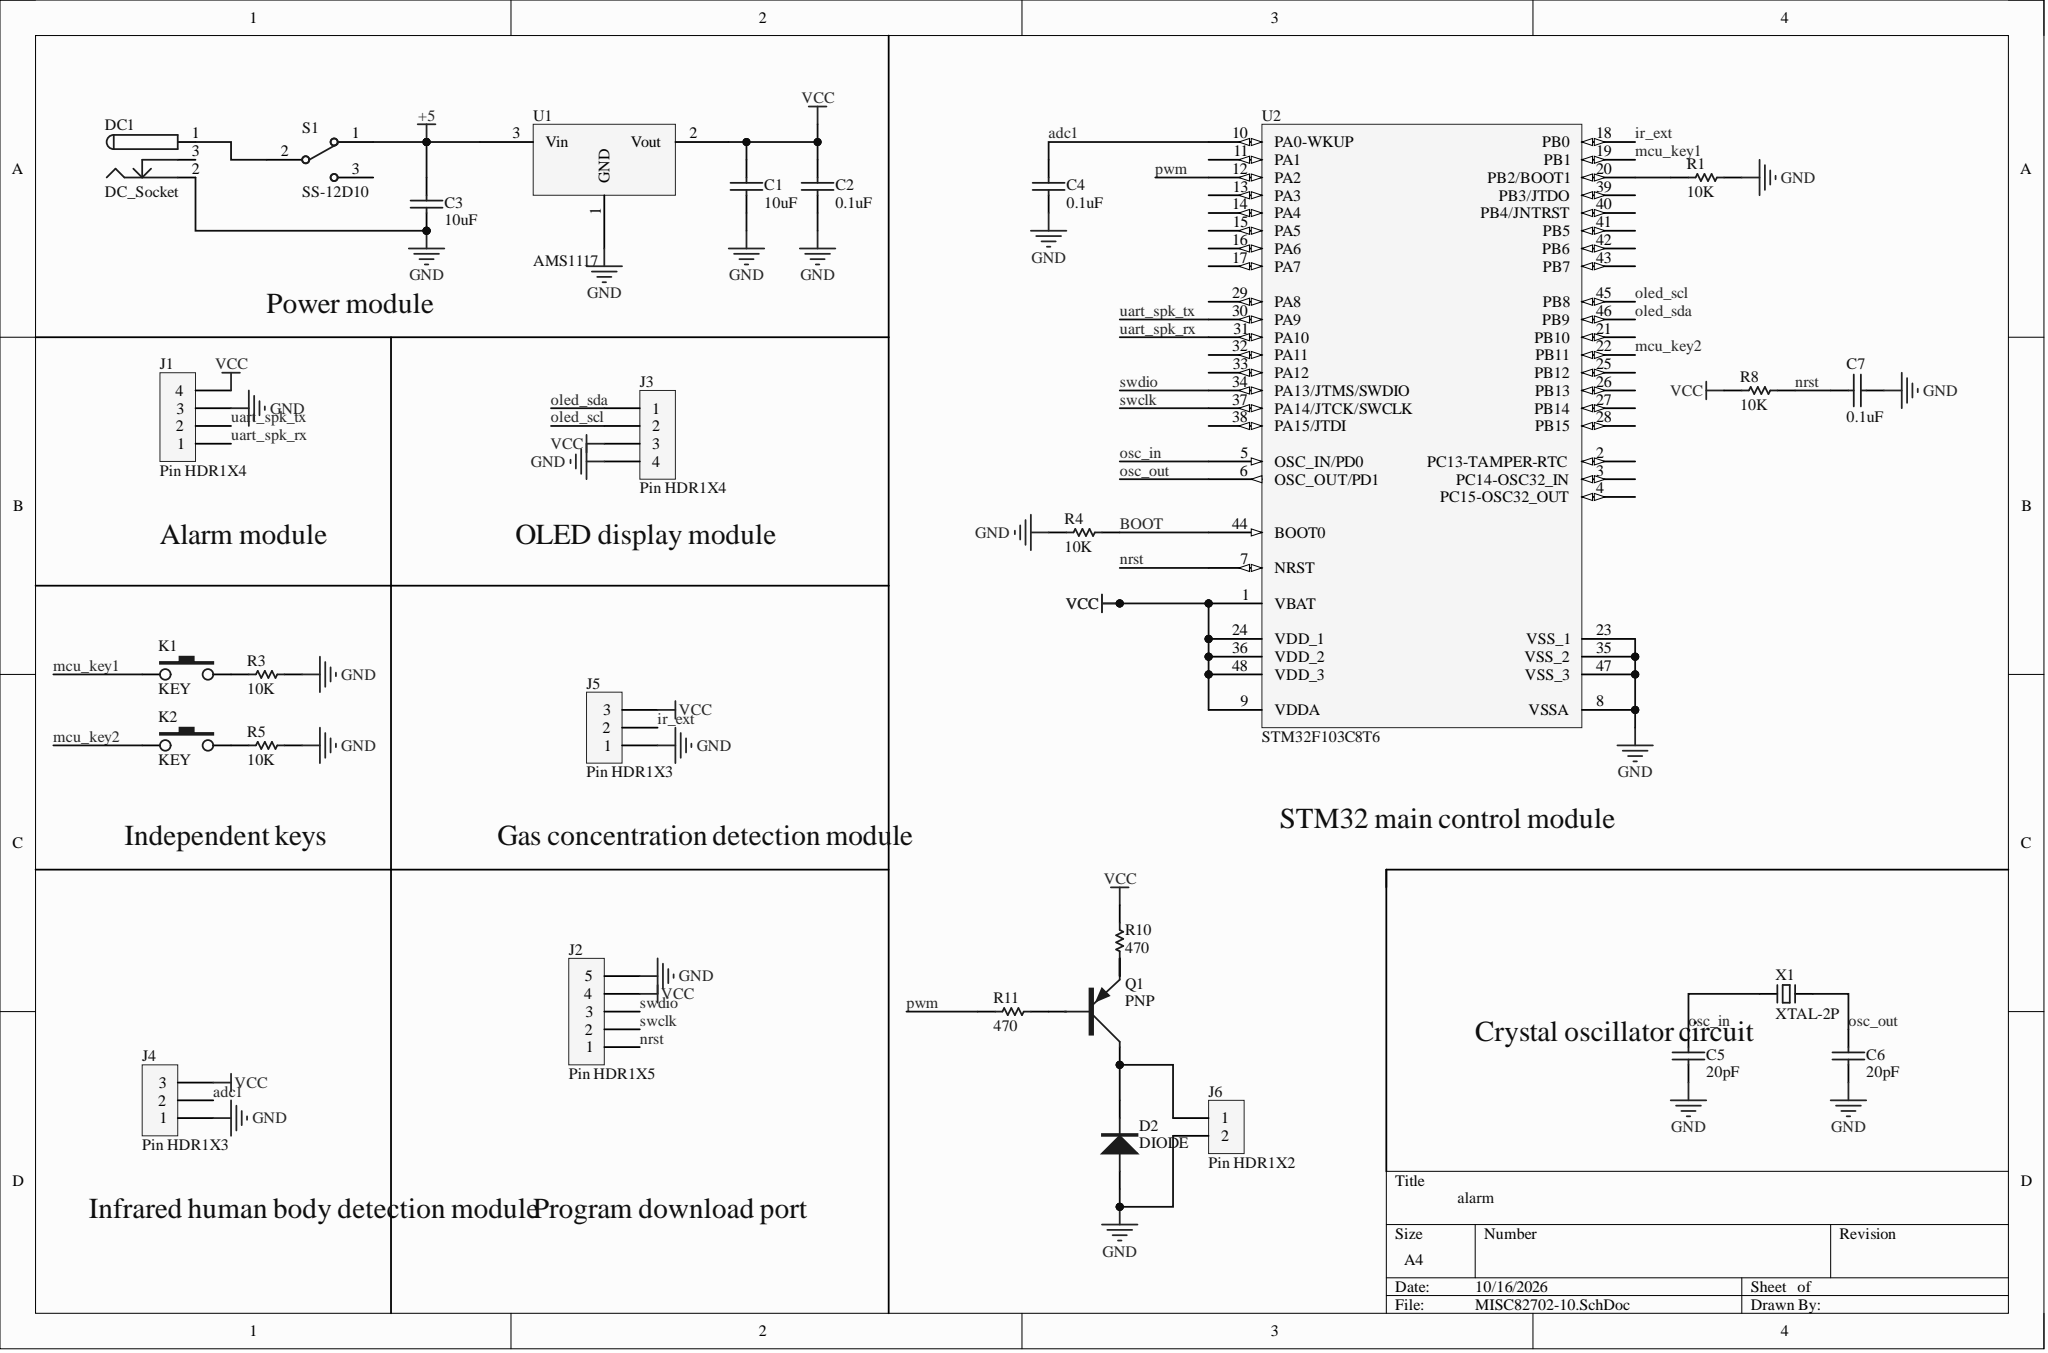Circuit board | Altium Designer | 29 parts | 25 nets
Bill of materials:
Comment,Description,Designator,Footprint,LibRef,Quantity
"10uF","Non-polar capacitor","C1, C3","0603C","CAP","2"
"0.1uF","Non-polar capacitor","C2, C4, C7","0603C","CAP","3"
"20pF","Non-polar capacitor","C5, C6","0603C","CAP","2"
"DIODE","General-purpose diode","D2","SOD-123","DIODE","1"
"DC_Socket","","DC1","DC-002","DC_Socket","1"
"Pin HDR1X4","","J1, J3","Pin HDR1X4/2.54mm-S","Pin HDR1X4","2"
"Pin HDR1X5","","J2","Pin HDR1X5/2.54mm-S","Pin HDR1X5","1"
"Pin HDR1X3","","J4, J5","Pin HDR1X3/2.54mm-S","Pin HDR1X3","2"
"Pin HDR1X2","","J6","Pin HDR1X2/2.54mm-S","Pin HDR1X2","1"
"KEY","","K1, K2","DIP-3X6X4.3","KEY","2"
"PNP","PNP transistor","Q1","SOT-23","PNP","1"
"10K","","R1, R3, R4, R5, R8","0603R","RES","5"
"470","","R10, R11","0603R","RES","2"
"SS-12D10","","S1","SS-12D10","SS-12D10","1"
"AMS1117","Three-terminal voltage regulator","U1","SOT223","AMS1117","1"
"STM32F103C8T6","","U2","LQFP48 7X7","STM32F103C8T6","1"
"XTAL-2P","2-pin passive crystal oscillator","X1","OSC HC-49S","XTAL-2P","1"
Netlist (Protel format):
[
C1
0603C
10uF



]
[
C2
0603C
0.1uF



]
[
C3
0603C
10uF



]
[
C4
0603C
0.1uF



]
[
C5
0603C
20pF



]
[
C6
0603C
20pF



]
[
C7
0603C
0.1uF



]
[
D2
SOD-123
DIODE



]
[
DC1
DC-002
DC_Socket



]
[
J1
Pin HDR1X4/2.54mm-S
Pin HDR1X4



]
[
J2
Pin HDR1X5/2.54mm-S
Pin HDR1X5



]
[
J3
Pin HDR1X4/2.54mm-S
Pin HDR1X4



]
[
J4
Pin HDR1X3/2.54mm-S
Pin HDR1X3



]
[
J5
Pin HDR1X3/2.54mm-S
Pin HDR1X3



]
[
J6
Pin HDR1X2/2.54mm-S
Pin HDR1X2



]
[
K1
DIP-3X6X4.3
KEY



]
[
K2
DIP-3X6X4.3
KEY



]
[
Q1
SOT-23
PNP



]
[
R1
0603R
10K



]
[
R3
0603R
10K



]
[
R4
0603R
10K



]
[
R5
0603R
10K



]
[
R8
0603R
10K



]
[
R10
0603R
470



]
[
R11
0603R
470



]
[
S1
SS-12D10
SS-12D10



]
[
U1
SOT223
AMS1117



]
[
U2
LQFP48 7X7
STM32F103C8T6



]
[
X1
OSC HC-49S
XTAL-2P



]
(
VCC
C1-2
C2-2
J1-4
J2-4
J3-3
J4-3
J5-3
R8-2
R10-1
U1-2
U2-1
U2-9
U2-24
U2-36
U2-48
)
(
uart_spk_tx
J1-2
U2-30
)
(
uart_spk_rx
J1-1
U2-31
)
(
swdio
J2-3
U2-34
)
(
swclk
J2-2
U2-37
)
(
pwm
R11-1
U2-12
)
(
osc_out
C6-2
U2-6
X1-2
)
(
osc_in
C5-2
U2-5
X1-1
)
(
oled_sda
J3-1
U2-46
)
(
oled_scl
J3-2
U2-45
)
(
nrst
C7-2
J2-1
R8-1
U2-7
)
(
NetR1_2
R1-2
U2-20
)
(
NetQ1_E
Q1-E
R10-2
)
(
NetQ1_B
Q1-B
R11-2
)
(
NetK2_3
K2-3
R5-2
)
(
NetK1_3
K1-3
R3-2
)
(
NetDC1_1
DC1-1
S1-2
)
(
NetD2_K
D2-K
J6-1
Q1-C
)
(
mcu_key2
K2-1
U2-22
)
(
mcu_key1
K1-1
U2-19
)
(
ir_ext
J5-2
U2-18
)
(
GND
C1-1
C2-1
C3-1
C4-1
C5-1
C6-1
C7-1
D2-A
DC1-2
J1-3
J2-5
J3-4
J4-1
J5-1
J6-2
R1-1
R3-1
R4-2
R5-1
U1-1
U2-8
U2-23
U2-35
U2-47
)
(
BOOT
R4-1
U2-44
)
(
adc1
C4-2
J4-2
U2-10
)
(
+5
C3-2
S1-1
U1-3
)